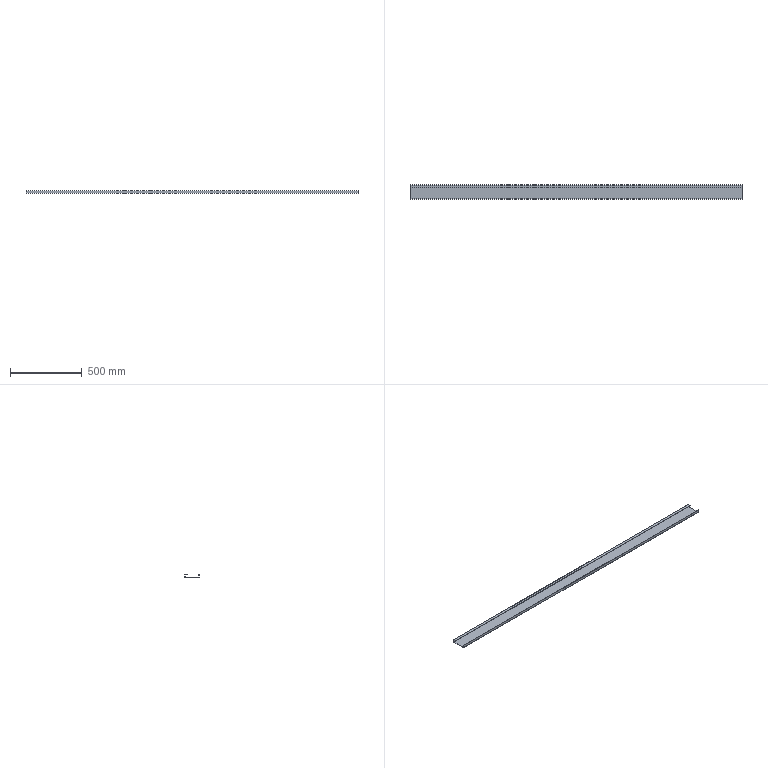Part | STEP file | 电柜通道护栏1踢脚Plate | 1 solid | 18 faces | box 2320 x 100 x 20 mm | volume 533298 mm3 | plane 12 | cylinder 6 | commonest cylinder face diameters 2 x3 5 x3
STEP:
#1=CARTESIAN_POINT('',(0.,0.,0.));
#2=DIRECTION('',(0.,0.,1.));
#3=DIRECTION('',(1.,0.,0.));
#4=AXIS2_PLACEMENT_3D('',#1,#2,#3);
#5=CARTESIAN_POINT('',(-1160.,1.5,2.5));
#6=VERTEX_POINT('',#5);
#7=CARTESIAN_POINT('',(-1160.,1.5,20.));
#8=VERTEX_POINT('',#7);
#9=CARTESIAN_POINT('',(-1160.,1.5,2.5));
#10=DIRECTION('',(0.,0.,1.));
#11=VECTOR('',#10,1.);
#12=LINE('',#9,#11);
#13=CARTESIAN_POINT('',(1160.,1.5,2.5));
#14=DIRECTION('',(0.,-1.,0.));
#15=DIRECTION('',(0.,0.,-1.));
#16=AXIS2_PLACEMENT_3D('',#13,#14,#15);
#17=PLANE('',#16);
#18=CARTESIAN_POINT('',(0.,-2320.));
#19=DIRECTION('',(-1.,0.));
#20=VECTOR('',#19,1.);
#21=LINE('',#18,#20);
#22=(GEOMETRIC_REPRESENTATION_CONTEXT(2)PARAMETRIC_REPRESENTATION_CONTEXT()REPRESENTATION_CONTEXT('',''));
#23=DEFINITIONAL_REPRESENTATION('',(#21),#22);
#24=PCURVE('',#17,#23);
#25=CARTESIAN_POINT('',(-1160.,2.5,2.5));
#26=DIRECTION('',(-1.,0.,0.));
#27=DIRECTION('',(0.,0.,1.));
#28=AXIS2_PLACEMENT_3D('',#25,#26,#27);
#29=PLANE('',#28);
#30=CARTESIAN_POINT('',(0.,-1.));
#31=DIRECTION('',(1.,0.));
#32=VECTOR('',#31,1.);
#33=LINE('',#30,#32);
#34=(GEOMETRIC_REPRESENTATION_CONTEXT(2)PARAMETRIC_REPRESENTATION_CONTEXT()REPRESENTATION_CONTEXT('',''));
#35=DEFINITIONAL_REPRESENTATION('',(#33),#34);
#36=PCURVE('',#29,#35);
#37=SURFACE_CURVE('',#12,(#24,#36),.PCURVE_S1.);
#38=EDGE_CURVE('',#6,#8,#37,.T.);
#39=ORIENTED_EDGE('',*,*,#38,.T.);
#40=CARTESIAN_POINT('',(1160.,1.5,20.));
#41=VERTEX_POINT('',#40);
#42=CARTESIAN_POINT('',(1160.,1.5,20.));
#43=DIRECTION('',(-1.,0.,0.));
#44=VECTOR('',#43,1.);
#45=LINE('',#42,#44);
#46=CARTESIAN_POINT('',(-17.5,0.));
#47=DIRECTION('',(0.,-1.));
#48=VECTOR('',#47,1.);
#49=LINE('',#46,#48);
#50=(GEOMETRIC_REPRESENTATION_CONTEXT(2)PARAMETRIC_REPRESENTATION_CONTEXT()REPRESENTATION_CONTEXT('',''));
#51=DEFINITIONAL_REPRESENTATION('',(#49),#50);
#52=PCURVE('',#17,#51);
#53=CARTESIAN_POINT('',(1160.,0.,20.));
#54=DIRECTION('',(0.,0.,1.));
#55=DIRECTION('',(1.,0.,0.));
#56=AXIS2_PLACEMENT_3D('',#53,#54,#55);
#57=PLANE('',#56);
#58=CARTESIAN_POINT('',(0.,1.5));
#59=DIRECTION('',(-1.,0.));
#60=VECTOR('',#59,1.);
#61=LINE('',#58,#60);
#62=(GEOMETRIC_REPRESENTATION_CONTEXT(2)PARAMETRIC_REPRESENTATION_CONTEXT()REPRESENTATION_CONTEXT('',''));
#63=DEFINITIONAL_REPRESENTATION('',(#61),#62);
#64=PCURVE('',#57,#63);
#65=SURFACE_CURVE('',#45,(#52,#64),.PCURVE_S1.);
#66=EDGE_CURVE('',#41,#8,#65,.T.);
#67=ORIENTED_EDGE('',*,*,#66,.F.);
#68=CARTESIAN_POINT('',(1160.,1.5,2.5));
#69=VERTEX_POINT('',#68);
#70=CARTESIAN_POINT('',(1160.,1.5,2.5));
#71=DIRECTION('',(0.,0.,1.));
#72=VECTOR('',#71,1.);
#73=LINE('',#70,#72);
#74=CARTESIAN_POINT('',(0.,0.));
#75=DIRECTION('',(-1.,0.));
#76=VECTOR('',#75,1.);
#77=LINE('',#74,#76);
#78=(GEOMETRIC_REPRESENTATION_CONTEXT(2)PARAMETRIC_REPRESENTATION_CONTEXT()REPRESENTATION_CONTEXT('',''));
#79=DEFINITIONAL_REPRESENTATION('',(#77),#78);
#80=PCURVE('',#17,#79);
#81=CARTESIAN_POINT('',(1160.,2.5,2.5));
#82=DIRECTION('',(-1.,0.,0.));
#83=DIRECTION('',(0.,0.,1.));
#84=AXIS2_PLACEMENT_3D('',#81,#82,#83);
#85=PLANE('',#84);
#86=CARTESIAN_POINT('',(0.,-1.));
#87=DIRECTION('',(1.,0.));
#88=VECTOR('',#87,1.);
#89=LINE('',#86,#88);
#90=(GEOMETRIC_REPRESENTATION_CONTEXT(2)PARAMETRIC_REPRESENTATION_CONTEXT()REPRESENTATION_CONTEXT('',''));
#91=DEFINITIONAL_REPRESENTATION('',(#89),#90);
#92=PCURVE('',#85,#91);
#93=SURFACE_CURVE('',#73,(#80,#92),.PCURVE_S1.);
#94=EDGE_CURVE('',#69,#41,#93,.T.);
#95=ORIENTED_EDGE('',*,*,#94,.F.);
#96=CARTESIAN_POINT('',(1160.,1.5,2.5));
#97=DIRECTION('',(-1.,0.,0.));
#98=VECTOR('',#97,1.);
#99=LINE('',#96,#98);
#100=CARTESIAN_POINT('',(0.,0.));
#101=DIRECTION('',(0.,-1.));
#102=VECTOR('',#101,1.);
#103=LINE('',#100,#102);
#104=(GEOMETRIC_REPRESENTATION_CONTEXT(2)PARAMETRIC_REPRESENTATION_CONTEXT()REPRESENTATION_CONTEXT('',''));
#105=DEFINITIONAL_REPRESENTATION('',(#103),#104);
#106=PCURVE('',#17,#105);
#107=CARTESIAN_POINT('',(1160.,2.5,2.5));
#108=DIRECTION('',(-1.,0.,0.));
#109=DIRECTION('',(0.,0.,1.));
#110=AXIS2_PLACEMENT_3D('',#107,#108,#109);
#111=CYLINDRICAL_SURFACE('',#110,1.);
#112=CARTESIAN_POINT('',(4.712,0.));
#113=DIRECTION('',(0.,1.));
#114=VECTOR('',#113,1.);
#115=LINE('',#112,#114);
#116=(GEOMETRIC_REPRESENTATION_CONTEXT(2)PARAMETRIC_REPRESENTATION_CONTEXT()REPRESENTATION_CONTEXT('',''));
#117=DEFINITIONAL_REPRESENTATION('',(#115),#116);
#118=PCURVE('',#111,#117);
#119=SURFACE_CURVE('',#99,(#106,#118),.PCURVE_S1.);
#120=EDGE_CURVE('',#69,#6,#119,.T.);
#121=ORIENTED_EDGE('',*,*,#120,.T.);
#122=EDGE_LOOP('',(#39,#67,#95,#121));
#123=FACE_BOUND('',#122,.T.);
#124=ADVANCED_FACE('',(#123),#17,.F.);
#125=CARTESIAN_POINT('',(-1160.,0.,20.));
#126=VERTEX_POINT('',#125);
#127=CARTESIAN_POINT('',(-1160.,0.,20.));
#128=DIRECTION('',(0.,1.,0.));
#129=VECTOR('',#128,1.);
#130=LINE('',#127,#129);
#131=CARTESIAN_POINT('',(-2320.,0.));
#132=DIRECTION('',(0.,1.));
#133=VECTOR('',#132,1.);
#134=LINE('',#131,#133);
#135=(GEOMETRIC_REPRESENTATION_CONTEXT(2)PARAMETRIC_REPRESENTATION_CONTEXT()REPRESENTATION_CONTEXT('',''));
#136=DEFINITIONAL_REPRESENTATION('',(#134),#135);
#137=PCURVE('',#57,#136);
#138=CARTESIAN_POINT('',(17.5,-2.5));
#139=DIRECTION('',(0.,1.));
#140=VECTOR('',#139,1.);
#141=LINE('',#138,#140);
#142=(GEOMETRIC_REPRESENTATION_CONTEXT(2)PARAMETRIC_REPRESENTATION_CONTEXT()REPRESENTATION_CONTEXT('',''));
#143=DEFINITIONAL_REPRESENTATION('',(#141),#142);
#144=PCURVE('',#29,#143);
#145=SURFACE_CURVE('',#130,(#137,#144),.PCURVE_S1.);
#146=EDGE_CURVE('',#126,#8,#145,.T.);
#147=ORIENTED_EDGE('',*,*,#146,.F.);
#148=CARTESIAN_POINT('',(1160.,0.,20.));
#149=VERTEX_POINT('',#148);
#150=CARTESIAN_POINT('',(1160.,0.,20.));
#151=DIRECTION('',(-1.,0.,0.));
#152=VECTOR('',#151,1.);
#153=LINE('',#150,#152);
#154=CARTESIAN_POINT('',(0.,0.));
#155=DIRECTION('',(-1.,0.));
#156=VECTOR('',#155,1.);
#157=LINE('',#154,#156);
#158=(GEOMETRIC_REPRESENTATION_CONTEXT(2)PARAMETRIC_REPRESENTATION_CONTEXT()REPRESENTATION_CONTEXT('',''));
#159=DEFINITIONAL_REPRESENTATION('',(#157),#158);
#160=PCURVE('',#57,#159);
#161=CARTESIAN_POINT('',(1160.,0.,2.5));
#162=DIRECTION('',(0.,-1.,0.));
#163=DIRECTION('',(0.,0.,-1.));
#164=AXIS2_PLACEMENT_3D('',#161,#162,#163);
#165=PLANE('',#164);
#166=CARTESIAN_POINT('',(-17.5,0.));
#167=DIRECTION('',(0.,-1.));
#168=VECTOR('',#167,1.);
#169=LINE('',#166,#168);
#170=(GEOMETRIC_REPRESENTATION_CONTEXT(2)PARAMETRIC_REPRESENTATION_CONTEXT()REPRESENTATION_CONTEXT('',''));
#171=DEFINITIONAL_REPRESENTATION('',(#169),#170);
#172=PCURVE('',#165,#171);
#173=SURFACE_CURVE('',#153,(#160,#172),.PCURVE_S1.);
#174=EDGE_CURVE('',#149,#126,#173,.T.);
#175=ORIENTED_EDGE('',*,*,#174,.F.);
#176=CARTESIAN_POINT('',(1160.,0.,20.));
#177=DIRECTION('',(0.,1.,0.));
#178=VECTOR('',#177,1.);
#179=LINE('',#176,#178);
#180=CARTESIAN_POINT('',(0.,0.));
#181=DIRECTION('',(0.,1.));
#182=VECTOR('',#181,1.);
#183=LINE('',#180,#182);
#184=(GEOMETRIC_REPRESENTATION_CONTEXT(2)PARAMETRIC_REPRESENTATION_CONTEXT()REPRESENTATION_CONTEXT('',''));
#185=DEFINITIONAL_REPRESENTATION('',(#183),#184);
#186=PCURVE('',#57,#185);
#187=CARTESIAN_POINT('',(17.5,-2.5));
#188=DIRECTION('',(0.,1.));
#189=VECTOR('',#188,1.);
#190=LINE('',#187,#189);
#191=(GEOMETRIC_REPRESENTATION_CONTEXT(2)PARAMETRIC_REPRESENTATION_CONTEXT()REPRESENTATION_CONTEXT('',''));
#192=DEFINITIONAL_REPRESENTATION('',(#190),#191);
#193=PCURVE('',#85,#192);
#194=SURFACE_CURVE('',#179,(#186,#193),.PCURVE_S1.);
#195=EDGE_CURVE('',#149,#41,#194,.T.);
#196=ORIENTED_EDGE('',*,*,#195,.T.);
#197=ORIENTED_EDGE('',*,*,#66,.T.);
#198=EDGE_LOOP('',(#147,#175,#196,#197));
#199=FACE_BOUND('',#198,.T.);
#200=ADVANCED_FACE('',(#199),#57,.T.);
#201=CARTESIAN_POINT('',(-1160.,0.,2.5));
#202=VERTEX_POINT('',#201);
#203=CARTESIAN_POINT('',(-1160.,0.,2.5));
#204=DIRECTION('',(0.,0.,1.));
#205=VECTOR('',#204,1.);
#206=LINE('',#203,#205);
#207=CARTESIAN_POINT('',(0.,-2320.));
#208=DIRECTION('',(-1.,0.));
#209=VECTOR('',#208,1.);
#210=LINE('',#207,#209);
#211=(GEOMETRIC_REPRESENTATION_CONTEXT(2)PARAMETRIC_REPRESENTATION_CONTEXT()REPRESENTATION_CONTEXT('',''));
#212=DEFINITIONAL_REPRESENTATION('',(#210),#211);
#213=PCURVE('',#165,#212);
#214=CARTESIAN_POINT('',(0.,-2.5));
#215=DIRECTION('',(1.,0.));
#216=VECTOR('',#215,1.);
#217=LINE('',#214,#216);
#218=(GEOMETRIC_REPRESENTATION_CONTEXT(2)PARAMETRIC_REPRESENTATION_CONTEXT()REPRESENTATION_CONTEXT('',''));
#219=DEFINITIONAL_REPRESENTATION('',(#217),#218);
#220=PCURVE('',#29,#219);
#221=SURFACE_CURVE('',#206,(#213,#220),.PCURVE_S1.);
#222=EDGE_CURVE('',#202,#126,#221,.T.);
#223=ORIENTED_EDGE('',*,*,#222,.F.);
#224=CARTESIAN_POINT('',(1160.,0.,2.5));
#225=VERTEX_POINT('',#224);
#226=CARTESIAN_POINT('',(1160.,0.,2.5));
#227=DIRECTION('',(-1.,0.,0.));
#228=VECTOR('',#227,1.);
#229=LINE('',#226,#228);
#230=CARTESIAN_POINT('',(0.,0.));
#231=DIRECTION('',(0.,-1.));
#232=VECTOR('',#231,1.);
#233=LINE('',#230,#232);
#234=(GEOMETRIC_REPRESENTATION_CONTEXT(2)PARAMETRIC_REPRESENTATION_CONTEXT()REPRESENTATION_CONTEXT('',''));
#235=DEFINITIONAL_REPRESENTATION('',(#233),#234);
#236=PCURVE('',#165,#235);
#237=CARTESIAN_POINT('',(1160.,2.5,2.5));
#238=DIRECTION('',(-1.,0.,0.));
#239=DIRECTION('',(0.,0.,1.));
#240=AXIS2_PLACEMENT_3D('',#237,#238,#239);
#241=CYLINDRICAL_SURFACE('',#240,2.5);
#242=CARTESIAN_POINT('',(4.712,0.));
#243=DIRECTION('',(0.,1.));
#244=VECTOR('',#243,1.);
#245=LINE('',#242,#244);
#246=(GEOMETRIC_REPRESENTATION_CONTEXT(2)PARAMETRIC_REPRESENTATION_CONTEXT()REPRESENTATION_CONTEXT('',''));
#247=DEFINITIONAL_REPRESENTATION('',(#245),#246);
#248=PCURVE('',#241,#247);
#249=SURFACE_CURVE('',#229,(#236,#248),.PCURVE_S1.);
#250=EDGE_CURVE('',#225,#202,#249,.T.);
#251=ORIENTED_EDGE('',*,*,#250,.F.);
#252=CARTESIAN_POINT('',(1160.,0.,2.5));
#253=DIRECTION('',(0.,0.,1.));
#254=VECTOR('',#253,1.);
#255=LINE('',#252,#254);
#256=CARTESIAN_POINT('',(0.,0.));
#257=DIRECTION('',(-1.,0.));
#258=VECTOR('',#257,1.);
#259=LINE('',#256,#258);
#260=(GEOMETRIC_REPRESENTATION_CONTEXT(2)PARAMETRIC_REPRESENTATION_CONTEXT()REPRESENTATION_CONTEXT('',''));
#261=DEFINITIONAL_REPRESENTATION('',(#259),#260);
#262=PCURVE('',#165,#261);
#263=CARTESIAN_POINT('',(0.,-2.5));
#264=DIRECTION('',(1.,0.));
#265=VECTOR('',#264,1.);
#266=LINE('',#263,#265);
#267=(GEOMETRIC_REPRESENTATION_CONTEXT(2)PARAMETRIC_REPRESENTATION_CONTEXT()REPRESENTATION_CONTEXT('',''));
#268=DEFINITIONAL_REPRESENTATION('',(#266),#267);
#269=PCURVE('',#85,#268);
#270=SURFACE_CURVE('',#255,(#262,#269),.PCURVE_S1.);
#271=EDGE_CURVE('',#225,#149,#270,.T.);
#272=ORIENTED_EDGE('',*,*,#271,.T.);
#273=ORIENTED_EDGE('',*,*,#174,.T.);
#274=EDGE_LOOP('',(#223,#251,#272,#273));
#275=FACE_BOUND('',#274,.T.);
#276=ADVANCED_FACE('',(#275),#165,.T.);
#277=CARTESIAN_POINT('',(-1160.,2.5,0.));
#278=VERTEX_POINT('',#277);
#279=CARTESIAN_POINT('',(-1160.,2.5,2.5));
#280=DIRECTION('',(-1.,0.,0.));
#281=DIRECTION('',(0.,0.,1.));
#282=AXIS2_PLACEMENT_3D('',#279,#280,#281);
#283=CIRCLE('',#282,2.5);
#284=CARTESIAN_POINT('',(0.,2320.));
#285=DIRECTION('',(1.,0.));
#286=VECTOR('',#285,1.);
#287=LINE('',#284,#286);
#288=(GEOMETRIC_REPRESENTATION_CONTEXT(2)PARAMETRIC_REPRESENTATION_CONTEXT()REPRESENTATION_CONTEXT('',''));
#289=DEFINITIONAL_REPRESENTATION('',(#287),#288);
#290=PCURVE('',#241,#289);
#291=CARTESIAN_POINT('',(0.,0.));
#292=DIRECTION('',(1.,0.));
#293=AXIS2_PLACEMENT_2D('',#291,#292);
#294=CIRCLE('',#293,2.5);
#295=(GEOMETRIC_REPRESENTATION_CONTEXT(2)PARAMETRIC_REPRESENTATION_CONTEXT()REPRESENTATION_CONTEXT('',''));
#296=DEFINITIONAL_REPRESENTATION('',(#294),#295);
#297=PCURVE('',#29,#296);
#298=SURFACE_CURVE('',#283,(#290,#297),.PCURVE_S1.);
#299=EDGE_CURVE('',#278,#202,#298,.T.);
#300=ORIENTED_EDGE('',*,*,#299,.F.);
#301=CARTESIAN_POINT('',(1160.,2.5,0.));
#302=VERTEX_POINT('',#301);
#303=CARTESIAN_POINT('',(1160.,2.5,0.));
#304=DIRECTION('',(-1.,0.,0.));
#305=VECTOR('',#304,1.);
#306=LINE('',#303,#305);
#307=CARTESIAN_POINT('',(3.142,0.));
#308=DIRECTION('',(0.,1.));
#309=VECTOR('',#308,1.);
#310=LINE('',#307,#309);
#311=(GEOMETRIC_REPRESENTATION_CONTEXT(2)PARAMETRIC_REPRESENTATION_CONTEXT()REPRESENTATION_CONTEXT('',''));
#312=DEFINITIONAL_REPRESENTATION('',(#310),#311);
#313=PCURVE('',#241,#312);
#314=CARTESIAN_POINT('',(1160.,2.5,0.));
#315=DIRECTION('',(0.,0.,-1.));
#316=DIRECTION('',(-1.,0.,0.));
#317=AXIS2_PLACEMENT_3D('',#314,#315,#316);
#318=PLANE('',#317);
#319=CARTESIAN_POINT('',(0.,0.));
#320=DIRECTION('',(1.,0.));
#321=VECTOR('',#320,1.);
#322=LINE('',#319,#321);
#323=(GEOMETRIC_REPRESENTATION_CONTEXT(2)PARAMETRIC_REPRESENTATION_CONTEXT()REPRESENTATION_CONTEXT('',''));
#324=DEFINITIONAL_REPRESENTATION('',(#322),#323);
#325=PCURVE('',#318,#324);
#326=SURFACE_CURVE('',#306,(#313,#325),.PCURVE_S1.);
#327=EDGE_CURVE('',#302,#278,#326,.T.);
#328=ORIENTED_EDGE('',*,*,#327,.F.);
#329=CARTESIAN_POINT('',(1160.,2.5,2.5));
#330=DIRECTION('',(-1.,0.,0.));
#331=DIRECTION('',(0.,0.,1.));
#332=AXIS2_PLACEMENT_3D('',#329,#330,#331);
#333=CIRCLE('',#332,2.5);
#334=CARTESIAN_POINT('',(0.,0.));
#335=DIRECTION('',(1.,0.));
#336=VECTOR('',#335,1.);
#337=LINE('',#334,#336);
#338=(GEOMETRIC_REPRESENTATION_CONTEXT(2)PARAMETRIC_REPRESENTATION_CONTEXT()REPRESENTATION_CONTEXT('',''));
#339=DEFINITIONAL_REPRESENTATION('',(#337),#338);
#340=PCURVE('',#241,#339);
#341=CARTESIAN_POINT('',(0.,0.));
#342=DIRECTION('',(1.,0.));
#343=AXIS2_PLACEMENT_2D('',#341,#342);
#344=CIRCLE('',#343,2.5);
#345=(GEOMETRIC_REPRESENTATION_CONTEXT(2)PARAMETRIC_REPRESENTATION_CONTEXT()REPRESENTATION_CONTEXT('',''));
#346=DEFINITIONAL_REPRESENTATION('',(#344),#345);
#347=PCURVE('',#85,#346);
#348=SURFACE_CURVE('',#333,(#340,#347),.PCURVE_S1.);
#349=EDGE_CURVE('',#302,#225,#348,.T.);
#350=ORIENTED_EDGE('',*,*,#349,.T.);
#351=ORIENTED_EDGE('',*,*,#250,.T.);
#352=EDGE_LOOP('',(#300,#328,#350,#351));
#353=FACE_BOUND('',#352,.T.);
#354=ADVANCED_FACE('',(#353),#241,.T.);
#355=CARTESIAN_POINT('',(-1160.,97.5,0.));
#356=VERTEX_POINT('',#355);
#357=CARTESIAN_POINT('',(-1160.,2.5,0.));
#358=DIRECTION('',(0.,-1.,0.));
#359=VECTOR('',#358,1.);
#360=LINE('',#357,#359);
#361=CARTESIAN_POINT('',(2320.,0.));
#362=DIRECTION('',(0.,-1.));
#363=VECTOR('',#362,1.);
#364=LINE('',#361,#363);
#365=(GEOMETRIC_REPRESENTATION_CONTEXT(2)PARAMETRIC_REPRESENTATION_CONTEXT()REPRESENTATION_CONTEXT('',''));
#366=DEFINITIONAL_REPRESENTATION('',(#364),#365);
#367=PCURVE('',#318,#366);
#368=CARTESIAN_POINT('',(-2.5,0.));
#369=DIRECTION('',(0.,-1.));
#370=VECTOR('',#369,1.);
#371=LINE('',#368,#370);
#372=(GEOMETRIC_REPRESENTATION_CONTEXT(2)PARAMETRIC_REPRESENTATION_CONTEXT()REPRESENTATION_CONTEXT('',''));
#373=DEFINITIONAL_REPRESENTATION('',(#371),#372);
#374=PCURVE('',#29,#373);
#375=SURFACE_CURVE('',#360,(#367,#374),.PCURVE_S1.);
#376=EDGE_CURVE('',#356,#278,#375,.T.);
#377=ORIENTED_EDGE('',*,*,#376,.F.);
#378=CARTESIAN_POINT('',(1160.,97.5,0.));
#379=VERTEX_POINT('',#378);
#380=CARTESIAN_POINT('',(1160.,97.5,0.));
#381=DIRECTION('',(-1.,0.,0.));
#382=VECTOR('',#381,1.);
#383=LINE('',#380,#382);
#384=CARTESIAN_POINT('',(0.,95.));
#385=DIRECTION('',(1.,0.));
#386=VECTOR('',#385,1.);
#387=LINE('',#384,#386);
#388=(GEOMETRIC_REPRESENTATION_CONTEXT(2)PARAMETRIC_REPRESENTATION_CONTEXT()REPRESENTATION_CONTEXT('',''));
#389=DEFINITIONAL_REPRESENTATION('',(#387),#388);
#390=PCURVE('',#318,#389);
#391=CARTESIAN_POINT('',(1160.,97.5,2.5));
#392=DIRECTION('',(-1.,0.,0.));
#393=DIRECTION('',(0.,0.,1.));
#394=AXIS2_PLACEMENT_3D('',#391,#392,#393);
#395=CYLINDRICAL_SURFACE('',#394,2.5);
#396=CARTESIAN_POINT('',(3.142,0.));
#397=DIRECTION('',(0.,1.));
#398=VECTOR('',#397,1.);
#399=LINE('',#396,#398);
#400=(GEOMETRIC_REPRESENTATION_CONTEXT(2)PARAMETRIC_REPRESENTATION_CONTEXT()REPRESENTATION_CONTEXT('',''));
#401=DEFINITIONAL_REPRESENTATION('',(#399),#400);
#402=PCURVE('',#395,#401);
#403=SURFACE_CURVE('',#383,(#390,#402),.PCURVE_S1.);
#404=EDGE_CURVE('',#379,#356,#403,.T.);
#405=ORIENTED_EDGE('',*,*,#404,.F.);
#406=CARTESIAN_POINT('',(1160.,2.5,0.));
#407=DIRECTION('',(0.,-1.,0.));
#408=VECTOR('',#407,1.);
#409=LINE('',#406,#408);
#410=CARTESIAN_POINT('',(0.,0.));
#411=DIRECTION('',(0.,-1.));
#412=VECTOR('',#411,1.);
#413=LINE('',#410,#412);
#414=(GEOMETRIC_REPRESENTATION_CONTEXT(2)PARAMETRIC_REPRESENTATION_CONTEXT()REPRESENTATION_CONTEXT('',''));
#415=DEFINITIONAL_REPRESENTATION('',(#413),#414);
#416=PCURVE('',#318,#415);
#417=CARTESIAN_POINT('',(-2.5,0.));
#418=DIRECTION('',(0.,-1.));
#419=VECTOR('',#418,1.);
#420=LINE('',#417,#419);
#421=(GEOMETRIC_REPRESENTATION_CONTEXT(2)PARAMETRIC_REPRESENTATION_CONTEXT()REPRESENTATION_CONTEXT('',''));
#422=DEFINITIONAL_REPRESENTATION('',(#420),#421);
#423=PCURVE('',#85,#422);
#424=SURFACE_CURVE('',#409,(#416,#423),.PCURVE_S1.);
#425=EDGE_CURVE('',#379,#302,#424,.T.);
#426=ORIENTED_EDGE('',*,*,#425,.T.);
#427=ORIENTED_EDGE('',*,*,#327,.T.);
#428=EDGE_LOOP('',(#377,#405,#426,#427));
#429=FACE_BOUND('',#428,.T.);
#430=ADVANCED_FACE('',(#429),#318,.T.);
#431=CARTESIAN_POINT('',(-1160.,100.,2.5));
#432=VERTEX_POINT('',#431);
#433=CARTESIAN_POINT('',(-1160.,97.5,2.5));
#434=DIRECTION('',(-1.,0.,0.));
#435=DIRECTION('',(0.,0.,-1.));
#436=AXIS2_PLACEMENT_3D('',#433,#434,#435);
#437=CIRCLE('',#436,2.5);
#438=CARTESIAN_POINT('',(-3.142,2320.));
#439=DIRECTION('',(1.,0.));
#440=VECTOR('',#439,1.);
#441=LINE('',#438,#440);
#442=(GEOMETRIC_REPRESENTATION_CONTEXT(2)PARAMETRIC_REPRESENTATION_CONTEXT()REPRESENTATION_CONTEXT('',''));
#443=DEFINITIONAL_REPRESENTATION('',(#441),#442);
#444=PCURVE('',#395,#443);
#445=CARTESIAN_POINT('',(0.,95.));
#446=DIRECTION('',(-1.,0.));
#447=AXIS2_PLACEMENT_2D('',#445,#446);
#448=CIRCLE('',#447,2.5);
#449=(GEOMETRIC_REPRESENTATION_CONTEXT(2)PARAMETRIC_REPRESENTATION_CONTEXT()REPRESENTATION_CONTEXT('',''));
#450=DEFINITIONAL_REPRESENTATION('',(#448),#449);
#451=PCURVE('',#29,#450);
#452=SURFACE_CURVE('',#437,(#444,#451),.PCURVE_S1.);
#453=EDGE_CURVE('',#432,#356,#452,.T.);
#454=ORIENTED_EDGE('',*,*,#453,.F.);
#455=CARTESIAN_POINT('',(1160.,100.,2.5));
#456=VERTEX_POINT('',#455);
#457=CARTESIAN_POINT('',(1160.,100.,2.5));
#458=DIRECTION('',(-1.,0.,0.));
#459=VECTOR('',#458,1.);
#460=LINE('',#457,#459);
#461=CARTESIAN_POINT('',(1.571,0.));
#462=DIRECTION('',(0.,1.));
#463=VECTOR('',#462,1.);
#464=LINE('',#461,#463);
#465=(GEOMETRIC_REPRESENTATION_CONTEXT(2)PARAMETRIC_REPRESENTATION_CONTEXT()REPRESENTATION_CONTEXT('',''));
#466=DEFINITIONAL_REPRESENTATION('',(#464),#465);
#467=PCURVE('',#395,#466);
#468=CARTESIAN_POINT('',(1160.,100.,2.5));
#469=DIRECTION('',(0.,1.,0.));
#470=DIRECTION('',(0.,0.,1.));
#471=AXIS2_PLACEMENT_3D('',#468,#469,#470);
#472=PLANE('',#471);
#473=CARTESIAN_POINT('',(0.,0.));
#474=DIRECTION('',(0.,-1.));
#475=VECTOR('',#474,1.);
#476=LINE('',#473,#475);
#477=(GEOMETRIC_REPRESENTATION_CONTEXT(2)PARAMETRIC_REPRESENTATION_CONTEXT()REPRESENTATION_CONTEXT('',''));
#478=DEFINITIONAL_REPRESENTATION('',(#476),#477);
#479=PCURVE('',#472,#478);
#480=SURFACE_CURVE('',#460,(#467,#479),.PCURVE_S1.);
#481=EDGE_CURVE('',#456,#432,#480,.T.);
#482=ORIENTED_EDGE('',*,*,#481,.F.);
#483=CARTESIAN_POINT('',(1160.,97.5,2.5));
#484=DIRECTION('',(-1.,0.,0.));
#485=DIRECTION('',(0.,0.,-1.));
#486=AXIS2_PLACEMENT_3D('',#483,#484,#485);
#487=CIRCLE('',#486,2.5);
#488=CARTESIAN_POINT('',(-3.142,0.));
#489=DIRECTION('',(1.,0.));
#490=VECTOR('',#489,1.);
#491=LINE('',#488,#490);
#492=(GEOMETRIC_REPRESENTATION_CONTEXT(2)PARAMETRIC_REPRESENTATION_CONTEXT()REPRESENTATION_CONTEXT('',''));
#493=DEFINITIONAL_REPRESENTATION('',(#491),#492);
#494=PCURVE('',#395,#493);
#495=CARTESIAN_POINT('',(0.,95.));
#496=DIRECTION('',(-1.,0.));
#497=AXIS2_PLACEMENT_2D('',#495,#496);
#498=CIRCLE('',#497,2.5);
#499=(GEOMETRIC_REPRESENTATION_CONTEXT(2)PARAMETRIC_REPRESENTATION_CONTEXT()REPRESENTATION_CONTEXT('',''));
#500=DEFINITIONAL_REPRESENTATION('',(#498),#499);
#501=PCURVE('',#85,#500);
#502=SURFACE_CURVE('',#487,(#494,#501),.PCURVE_S1.);
#503=EDGE_CURVE('',#456,#379,#502,.T.);
#504=ORIENTED_EDGE('',*,*,#503,.T.);
#505=ORIENTED_EDGE('',*,*,#404,.T.);
#506=EDGE_LOOP('',(#454,#482,#504,#505));
#507=FACE_BOUND('',#506,.T.);
#508=ADVANCED_FACE('',(#507),#395,.T.);
#509=CARTESIAN_POINT('',(-1160.,100.,17.5));
#510=VERTEX_POINT('',#509);
#511=CARTESIAN_POINT('',(-1160.,100.,2.5));
#512=DIRECTION('',(0.,0.,-1.));
#513=VECTOR('',#512,1.);
#514=LINE('',#511,#513);
#515=CARTESIAN_POINT('',(0.,-2320.));
#516=DIRECTION('',(-1.,0.));
#517=VECTOR('',#516,1.);
#518=LINE('',#515,#517);
#519=(GEOMETRIC_REPRESENTATION_CONTEXT(2)PARAMETRIC_REPRESENTATION_CONTEXT()REPRESENTATION_CONTEXT('',''));
#520=DEFINITIONAL_REPRESENTATION('',(#518),#519);
#521=PCURVE('',#472,#520);
#522=CARTESIAN_POINT('',(0.,97.5));
#523=DIRECTION('',(-1.,0.));
#524=VECTOR('',#523,1.);
#525=LINE('',#522,#524);
#526=(GEOMETRIC_REPRESENTATION_CONTEXT(2)PARAMETRIC_REPRESENTATION_CONTEXT()REPRESENTATION_CONTEXT('',''));
#527=DEFINITIONAL_REPRESENTATION('',(#525),#526);
#528=PCURVE('',#29,#527);
#529=SURFACE_CURVE('',#514,(#521,#528),.PCURVE_S1.);
#530=EDGE_CURVE('',#510,#432,#529,.T.);
#531=ORIENTED_EDGE('',*,*,#530,.F.);
#532=CARTESIAN_POINT('',(1160.,100.,17.5));
#533=VERTEX_POINT('',#532);
#534=CARTESIAN_POINT('',(1160.,100.,17.5));
#535=DIRECTION('',(-1.,0.,0.));
#536=VECTOR('',#535,1.);
#537=LINE('',#534,#536);
#538=CARTESIAN_POINT('',(15.,0.));
#539=DIRECTION('',(0.,-1.));
#540=VECTOR('',#539,1.);
#541=LINE('',#538,#540);
#542=(GEOMETRIC_REPRESENTATION_CONTEXT(2)PARAMETRIC_REPRESENTATION_CONTEXT()REPRESENTATION_CONTEXT('',''));
#543=DEFINITIONAL_REPRESENTATION('',(#541),#542);
#544=PCURVE('',#472,#543);
#545=CARTESIAN_POINT('',(1160.,97.5,17.5));
#546=DIRECTION('',(-1.,0.,0.));
#547=DIRECTION('',(0.,0.,1.));
#548=AXIS2_PLACEMENT_3D('',#545,#546,#547);
#549=CYLINDRICAL_SURFACE('',#548,2.5);
#550=CARTESIAN_POINT('',(1.571,0.));
#551=DIRECTION('',(0.,1.));
#552=VECTOR('',#551,1.);
#553=LINE('',#550,#552);
#554=(GEOMETRIC_REPRESENTATION_CONTEXT(2)PARAMETRIC_REPRESENTATION_CONTEXT()REPRESENTATION_CONTEXT('',''));
#555=DEFINITIONAL_REPRESENTATION('',(#553),#554);
#556=PCURVE('',#549,#555);
#557=SURFACE_CURVE('',#537,(#544,#556),.PCURVE_S1.);
#558=EDGE_CURVE('',#533,#510,#557,.T.);
#559=ORIENTED_EDGE('',*,*,#558,.F.);
#560=CARTESIAN_POINT('',(1160.,100.,2.5));
#561=DIRECTION('',(0.,0.,-1.));
#562=VECTOR('',#561,1.);
#563=LINE('',#560,#562);
#564=CARTESIAN_POINT('',(0.,0.));
#565=DIRECTION('',(-1.,0.));
#566=VECTOR('',#565,1.);
#567=LINE('',#564,#566);
#568=(GEOMETRIC_REPRESENTATION_CONTEXT(2)PARAMETRIC_REPRESENTATION_CONTEXT()REPRESENTATION_CONTEXT('',''));
#569=DEFINITIONAL_REPRESENTATION('',(#567),#568);
#570=PCURVE('',#472,#569);
#571=CARTESIAN_POINT('',(0.,97.5));
#572=DIRECTION('',(-1.,0.));
#573=VECTOR('',#572,1.);
#574=LINE('',#571,#573);
#575=(GEOMETRIC_REPRESENTATION_CONTEXT(2)PARAMETRIC_REPRESENTATION_CONTEXT()REPRESENTATION_CONTEXT('',''));
#576=DEFINITIONAL_REPRESENTATION('',(#574),#575);
#577=PCURVE('',#85,#576);
#578=SURFACE_CURVE('',#563,(#570,#577),.PCURVE_S1.);
#579=EDGE_CURVE('',#533,#456,#578,.T.);
#580=ORIENTED_EDGE('',*,*,#579,.T.);
#581=ORIENTED_EDGE('',*,*,#481,.T.);
#582=EDGE_LOOP('',(#531,#559,#580,#581));
#583=FACE_BOUND('',#582,.T.);
#584=ADVANCED_FACE('',(#583),#472,.T.);
#585=CARTESIAN_POINT('',(-1160.,97.5,20.));
#586=VERTEX_POINT('',#585);
#587=CARTESIAN_POINT('',(-1160.,97.5,17.5));
#588=DIRECTION('',(-1.,0.,0.));
#589=DIRECTION('',(0.,0.,-1.));
#590=AXIS2_PLACEMENT_3D('',#587,#588,#589);
#591=CIRCLE('',#590,2.5);
#592=CARTESIAN_POINT('',(-3.142,2320.));
#593=DIRECTION('',(1.,0.));
#594=VECTOR('',#593,1.);
#595=LINE('',#592,#594);
#596=(GEOMETRIC_REPRESENTATION_CONTEXT(2)PARAMETRIC_REPRESENTATION_CONTEXT()REPRESENTATION_CONTEXT('',''));
#597=DEFINITIONAL_REPRESENTATION('',(#595),#596);
#598=PCURVE('',#549,#597);
#599=CARTESIAN_POINT('',(15.,95.));
#600=DIRECTION('',(-1.,0.));
#601=AXIS2_PLACEMENT_2D('',#599,#600);
#602=CIRCLE('',#601,2.5);
#603=(GEOMETRIC_REPRESENTATION_CONTEXT(2)PARAMETRIC_REPRESENTATION_CONTEXT()REPRESENTATION_CONTEXT('',''));
#604=DEFINITIONAL_REPRESENTATION('',(#602),#603);
#605=PCURVE('',#29,#604);
#606=SURFACE_CURVE('',#591,(#598,#605),.PCURVE_S1.);
#607=EDGE_CURVE('',#586,#510,#606,.T.);
#608=ORIENTED_EDGE('',*,*,#607,.F.);
#609=CARTESIAN_POINT('',(1160.,97.5,20.));
#610=VERTEX_POINT('',#609);
#611=CARTESIAN_POINT('',(1160.,97.5,20.));
#612=DIRECTION('',(-1.,0.,0.));
#613=VECTOR('',#612,1.);
#614=LINE('',#611,#613);
#615=CARTESIAN_POINT('',(0.,0.));
#616=DIRECTION('',(0.,1.));
#617=VECTOR('',#616,1.);
#618=LINE('',#615,#617);
#619=(GEOMETRIC_REPRESENTATION_CONTEXT(2)PARAMETRIC_REPRESENTATION_CONTEXT()REPRESENTATION_CONTEXT('',''));
#620=DEFINITIONAL_REPRESENTATION('',(#618),#619);
#621=PCURVE('',#549,#620);
#622=CARTESIAN_POINT('',(1160.,97.5,20.));
#623=DIRECTION('',(0.,0.,1.));
#624=DIRECTION('',(1.,0.,0.));
#625=AXIS2_PLACEMENT_3D('',#622,#623,#624);
#626=PLANE('',#625);
#627=CARTESIAN_POINT('',(0.,0.));
#628=DIRECTION('',(-1.,0.));
#629=VECTOR('',#628,1.);
#630=LINE('',#627,#629);
#631=(GEOMETRIC_REPRESENTATION_CONTEXT(2)PARAMETRIC_REPRESENTATION_CONTEXT()REPRESENTATION_CONTEXT('',''));
#632=DEFINITIONAL_REPRESENTATION('',(#630),#631);
#633=PCURVE('',#626,#632);
#634=SURFACE_CURVE('',#614,(#621,#633),.PCURVE_S1.);
#635=EDGE_CURVE('',#610,#586,#634,.T.);
#636=ORIENTED_EDGE('',*,*,#635,.F.);
#637=CARTESIAN_POINT('',(1160.,97.5,17.5));
#638=DIRECTION('',(-1.,0.,0.));
#639=DIRECTION('',(0.,0.,-1.));
#640=AXIS2_PLACEMENT_3D('',#637,#638,#639);
#641=CIRCLE('',#640,2.5);
#642=CARTESIAN_POINT('',(-3.142,0.));
#643=DIRECTION('',(1.,0.));
#644=VECTOR('',#643,1.);
#645=LINE('',#642,#644);
#646=(GEOMETRIC_REPRESENTATION_CONTEXT(2)PARAMETRIC_REPRESENTATION_CONTEXT()REPRESENTATION_CONTEXT('',''));
#647=DEFINITIONAL_REPRESENTATION('',(#645),#646);
#648=PCURVE('',#549,#647);
#649=CARTESIAN_POINT('',(15.,95.));
#650=DIRECTION('',(-1.,0.));
#651=AXIS2_PLACEMENT_2D('',#649,#650);
#652=CIRCLE('',#651,2.5);
#653=(GEOMETRIC_REPRESENTATION_CONTEXT(2)PARAMETRIC_REPRESENTATION_CONTEXT()REPRESENTATION_CONTEXT('',''));
#654=DEFINITIONAL_REPRESENTATION('',(#652),#653);
#655=PCURVE('',#85,#654);
#656=SURFACE_CURVE('',#641,(#648,#655),.PCURVE_S1.);
#657=EDGE_CURVE('',#610,#533,#656,.T.);
#658=ORIENTED_EDGE('',*,*,#657,.T.);
#659=ORIENTED_EDGE('',*,*,#558,.T.);
#660=EDGE_LOOP('',(#608,#636,#658,#659));
#661=FACE_BOUND('',#660,.T.);
#662=ADVANCED_FACE('',(#661),#549,.T.);
#663=CARTESIAN_POINT('',(-1160.,80.,20.));
#664=VERTEX_POINT('',#663);
#665=CARTESIAN_POINT('',(-1160.,97.5,20.));
#666=DIRECTION('',(0.,1.,0.));
#667=VECTOR('',#666,1.);
#668=LINE('',#665,#667);
#669=CARTESIAN_POINT('',(-2320.,0.));
#670=DIRECTION('',(0.,1.));
#671=VECTOR('',#670,1.);
#672=LINE('',#669,#671);
#673=(GEOMETRIC_REPRESENTATION_CONTEXT(2)PARAMETRIC_REPRESENTATION_CONTEXT()REPRESENTATION_CONTEXT('',''));
#674=DEFINITIONAL_REPRESENTATION('',(#672),#673);
#675=PCURVE('',#626,#674);
#676=CARTESIAN_POINT('',(17.5,95.));
#677=DIRECTION('',(0.,1.));
#678=VECTOR('',#677,1.);
#679=LINE('',#676,#678);
#680=(GEOMETRIC_REPRESENTATION_CONTEXT(2)PARAMETRIC_REPRESENTATION_CONTEXT()REPRESENTATION_CONTEXT('',''));
#681=DEFINITIONAL_REPRESENTATION('',(#679),#680);
#682=PCURVE('',#29,#681);
#683=SURFACE_CURVE('',#668,(#675,#682),.PCURVE_S1.);
#684=EDGE_CURVE('',#664,#586,#683,.T.);
#685=ORIENTED_EDGE('',*,*,#684,.F.);
#686=CARTESIAN_POINT('',(1160.,80.,20.));
#687=VERTEX_POINT('',#686);
#688=CARTESIAN_POINT('',(1160.,80.,20.));
#689=DIRECTION('',(-1.,0.,0.));
#690=VECTOR('',#689,1.);
#691=LINE('',#688,#690);
#692=CARTESIAN_POINT('',(0.,-17.5));
#693=DIRECTION('',(-1.,0.));
#694=VECTOR('',#693,1.);
#695=LINE('',#692,#694);
#696=(GEOMETRIC_REPRESENTATION_CONTEXT(2)PARAMETRIC_REPRESENTATION_CONTEXT()REPRESENTATION_CONTEXT('',''));
#697=DEFINITIONAL_REPRESENTATION('',(#695),#696);
#698=PCURVE('',#626,#697);
#699=CARTESIAN_POINT('',(1160.,80.,18.5));
#700=DIRECTION('',(0.,-1.,0.));
#701=DIRECTION('',(0.,0.,-1.));
#702=AXIS2_PLACEMENT_3D('',#699,#700,#701);
#703=PLANE('',#702);
#704=CARTESIAN_POINT('',(-1.5,0.));
#705=DIRECTION('',(0.,-1.));
#706=VECTOR('',#705,1.);
#707=LINE('',#704,#706);
#708=(GEOMETRIC_REPRESENTATION_CONTEXT(2)PARAMETRIC_REPRESENTATION_CONTEXT()REPRESENTATION_CONTEXT('',''));
#709=DEFINITIONAL_REPRESENTATION('',(#707),#708);
#710=PCURVE('',#703,#709);
#711=SURFACE_CURVE('',#691,(#698,#710),.PCURVE_S1.);
#712=EDGE_CURVE('',#687,#664,#711,.T.);
#713=ORIENTED_EDGE('',*,*,#712,.F.);
#714=CARTESIAN_POINT('',(1160.,97.5,20.));
#715=DIRECTION('',(0.,1.,0.));
#716=VECTOR('',#715,1.);
#717=LINE('',#714,#716);
#718=CARTESIAN_POINT('',(0.,0.));
#719=DIRECTION('',(0.,1.));
#720=VECTOR('',#719,1.);
#721=LINE('',#718,#720);
#722=(GEOMETRIC_REPRESENTATION_CONTEXT(2)PARAMETRIC_REPRESENTATION_CONTEXT()REPRESENTATION_CONTEXT('',''));
#723=DEFINITIONAL_REPRESENTATION('',(#721),#722);
#724=PCURVE('',#626,#723);
#725=CARTESIAN_POINT('',(17.5,95.));
#726=DIRECTION('',(0.,1.));
#727=VECTOR('',#726,1.);
#728=LINE('',#725,#727);
#729=(GEOMETRIC_REPRESENTATION_CONTEXT(2)PARAMETRIC_REPRESENTATION_CONTEXT()REPRESENTATION_CONTEXT('',''));
#730=DEFINITIONAL_REPRESENTATION('',(#728),#729);
#731=PCURVE('',#85,#730);
#732=SURFACE_CURVE('',#717,(#724,#731),.PCURVE_S1.);
#733=EDGE_CURVE('',#687,#610,#732,.T.);
#734=ORIENTED_EDGE('',*,*,#733,.T.);
#735=ORIENTED_EDGE('',*,*,#635,.T.);
#736=EDGE_LOOP('',(#685,#713,#734,#735));
#737=FACE_BOUND('',#736,.T.);
#738=ADVANCED_FACE('',(#737),#626,.T.);
#739=CARTESIAN_POINT('',(-1160.,80.,18.5));
#740=VERTEX_POINT('',#739);
#741=CARTESIAN_POINT('',(-1160.,80.,18.5));
#742=DIRECTION('',(0.,0.,1.));
#743=VECTOR('',#742,1.);
#744=LINE('',#741,#743);
#745=CARTESIAN_POINT('',(0.,-2320.));
#746=DIRECTION('',(-1.,0.));
#747=VECTOR('',#746,1.);
#748=LINE('',#745,#747);
#749=(GEOMETRIC_REPRESENTATION_CONTEXT(2)PARAMETRIC_REPRESENTATION_CONTEXT()REPRESENTATION_CONTEXT('',''));
#750=DEFINITIONAL_REPRESENTATION('',(#748),#749);
#751=PCURVE('',#703,#750);
#752=CARTESIAN_POINT('',(16.,77.5));
#753=DIRECTION('',(1.,0.));
#754=VECTOR('',#753,1.);
#755=LINE('',#752,#754);
#756=(GEOMETRIC_REPRESENTATION_CONTEXT(2)PARAMETRIC_REPRESENTATION_CONTEXT()REPRESENTATION_CONTEXT('',''));
#757=DEFINITIONAL_REPRESENTATION('',(#755),#756);
#758=PCURVE('',#29,#757);
#759=SURFACE_CURVE('',#744,(#751,#758),.PCURVE_S1.);
#760=EDGE_CURVE('',#740,#664,#759,.T.);
#761=ORIENTED_EDGE('',*,*,#760,.F.);
#762=CARTESIAN_POINT('',(1160.,80.,18.5));
#763=VERTEX_POINT('',#762);
#764=CARTESIAN_POINT('',(1160.,80.,18.5));
#765=DIRECTION('',(-1.,0.,0.));
#766=VECTOR('',#765,1.);
#767=LINE('',#764,#766);
#768=CARTESIAN_POINT('',(0.,0.));
#769=DIRECTION('',(0.,-1.));
#770=VECTOR('',#769,1.);
#771=LINE('',#768,#770);
#772=(GEOMETRIC_REPRESENTATION_CONTEXT(2)PARAMETRIC_REPRESENTATION_CONTEXT()REPRESENTATION_CONTEXT('',''));
#773=DEFINITIONAL_REPRESENTATION('',(#771),#772);
#774=PCURVE('',#703,#773);
#775=CARTESIAN_POINT('',(1160.,97.5,18.5));
#776=DIRECTION('',(0.,0.,1.));
#777=DIRECTION('',(1.,0.,0.));
#778=AXIS2_PLACEMENT_3D('',#775,#776,#777);
#779=PLANE('',#778);
#780=CARTESIAN_POINT('',(0.,-17.5));
#781=DIRECTION('',(-1.,0.));
#782=VECTOR('',#781,1.);
#783=LINE('',#780,#782);
#784=(GEOMETRIC_REPRESENTATION_CONTEXT(2)PARAMETRIC_REPRESENTATION_CONTEXT()REPRESENTATION_CONTEXT('',''));
#785=DEFINITIONAL_REPRESENTATION('',(#783),#784);
#786=PCURVE('',#779,#785);
#787=SURFACE_CURVE('',#767,(#774,#786),.PCURVE_S1.);
#788=EDGE_CURVE('',#763,#740,#787,.T.);
#789=ORIENTED_EDGE('',*,*,#788,.F.);
#790=CARTESIAN_POINT('',(1160.,80.,18.5));
#791=DIRECTION('',(0.,0.,1.));
#792=VECTOR('',#791,1.);
#793=LINE('',#790,#792);
#794=CARTESIAN_POINT('',(0.,0.));
#795=DIRECTION('',(-1.,0.));
#796=VECTOR('',#795,1.);
#797=LINE('',#794,#796);
#798=(GEOMETRIC_REPRESENTATION_CONTEXT(2)PARAMETRIC_REPRESENTATION_CONTEXT()REPRESENTATION_CONTEXT('',''));
#799=DEFINITIONAL_REPRESENTATION('',(#797),#798);
#800=PCURVE('',#703,#799);
#801=CARTESIAN_POINT('',(16.,77.5));
#802=DIRECTION('',(1.,0.));
#803=VECTOR('',#802,1.);
#804=LINE('',#801,#803);
#805=(GEOMETRIC_REPRESENTATION_CONTEXT(2)PARAMETRIC_REPRESENTATION_CONTEXT()REPRESENTATION_CONTEXT('',''));
#806=DEFINITIONAL_REPRESENTATION('',(#804),#805);
#807=PCURVE('',#85,#806);
#808=SURFACE_CURVE('',#793,(#800,#807),.PCURVE_S1.);
#809=EDGE_CURVE('',#763,#687,#808,.T.);
#810=ORIENTED_EDGE('',*,*,#809,.T.);
#811=ORIENTED_EDGE('',*,*,#712,.T.);
#812=EDGE_LOOP('',(#761,#789,#810,#811));
#813=FACE_BOUND('',#812,.T.);
#814=ADVANCED_FACE('',(#813),#703,.T.);
#815=CARTESIAN_POINT('',(-1160.,97.5,18.5));
#816=VERTEX_POINT('',#815);
#817=CARTESIAN_POINT('',(-1160.,97.5,18.5));
#818=DIRECTION('',(0.,1.,0.));
#819=VECTOR('',#818,1.);
#820=LINE('',#817,#819);
#821=CARTESIAN_POINT('',(-2320.,0.));
#822=DIRECTION('',(0.,1.));
#823=VECTOR('',#822,1.);
#824=LINE('',#821,#823);
#825=(GEOMETRIC_REPRESENTATION_CONTEXT(2)PARAMETRIC_REPRESENTATION_CONTEXT()REPRESENTATION_CONTEXT('',''));
#826=DEFINITIONAL_REPRESENTATION('',(#824),#825);
#827=PCURVE('',#779,#826);
#828=CARTESIAN_POINT('',(16.,95.));
#829=DIRECTION('',(0.,1.));
#830=VECTOR('',#829,1.);
#831=LINE('',#828,#830);
#832=(GEOMETRIC_REPRESENTATION_CONTEXT(2)PARAMETRIC_REPRESENTATION_CONTEXT()REPRESENTATION_CONTEXT('',''));
#833=DEFINITIONAL_REPRESENTATION('',(#831),#832);
#834=PCURVE('',#29,#833);
#835=SURFACE_CURVE('',#820,(#827,#834),.PCURVE_S1.);
#836=EDGE_CURVE('',#740,#816,#835,.T.);
#837=ORIENTED_EDGE('',*,*,#836,.T.);
#838=CARTESIAN_POINT('',(1160.,97.5,18.5));
#839=VERTEX_POINT('',#838);
#840=CARTESIAN_POINT('',(1160.,97.5,18.5));
#841=DIRECTION('',(-1.,0.,0.));
#842=VECTOR('',#841,1.);
#843=LINE('',#840,#842);
#844=CARTESIAN_POINT('',(0.,0.));
#845=DIRECTION('',(-1.,0.));
#846=VECTOR('',#845,1.);
#847=LINE('',#844,#846);
#848=(GEOMETRIC_REPRESENTATION_CONTEXT(2)PARAMETRIC_REPRESENTATION_CONTEXT()REPRESENTATION_CONTEXT('',''));
#849=DEFINITIONAL_REPRESENTATION('',(#847),#848);
#850=PCURVE('',#779,#849);
#851=CARTESIAN_POINT('',(1160.,97.5,17.5));
#852=DIRECTION('',(-1.,0.,0.));
#853=DIRECTION('',(0.,0.,1.));
#854=AXIS2_PLACEMENT_3D('',#851,#852,#853);
#855=CYLINDRICAL_SURFACE('',#854,1.);
#856=CARTESIAN_POINT('',(0.,0.));
#857=DIRECTION('',(0.,1.));
#858=VECTOR('',#857,1.);
#859=LINE('',#856,#858);
#860=(GEOMETRIC_REPRESENTATION_CONTEXT(2)PARAMETRIC_REPRESENTATION_CONTEXT()REPRESENTATION_CONTEXT('',''));
#861=DEFINITIONAL_REPRESENTATION('',(#859),#860);
#862=PCURVE('',#855,#861);
#863=SURFACE_CURVE('',#843,(#850,#862),.PCURVE_S1.);
#864=EDGE_CURVE('',#839,#816,#863,.T.);
#865=ORIENTED_EDGE('',*,*,#864,.F.);
#866=CARTESIAN_POINT('',(1160.,97.5,18.5));
#867=DIRECTION('',(0.,1.,0.));
#868=VECTOR('',#867,1.);
#869=LINE('',#866,#868);
#870=CARTESIAN_POINT('',(0.,0.));
#871=DIRECTION('',(0.,1.));
#872=VECTOR('',#871,1.);
#873=LINE('',#870,#872);
#874=(GEOMETRIC_REPRESENTATION_CONTEXT(2)PARAMETRIC_REPRESENTATION_CONTEXT()REPRESENTATION_CONTEXT('',''));
#875=DEFINITIONAL_REPRESENTATION('',(#873),#874);
#876=PCURVE('',#779,#875);
#877=CARTESIAN_POINT('',(16.,95.));
#878=DIRECTION('',(0.,1.));
#879=VECTOR('',#878,1.);
#880=LINE('',#877,#879);
#881=(GEOMETRIC_REPRESENTATION_CONTEXT(2)PARAMETRIC_REPRESENTATION_CONTEXT()REPRESENTATION_CONTEXT('',''));
#882=DEFINITIONAL_REPRESENTATION('',(#880),#881);
#883=PCURVE('',#85,#882);
#884=SURFACE_CURVE('',#869,(#876,#883),.PCURVE_S1.);
#885=EDGE_CURVE('',#763,#839,#884,.T.);
#886=ORIENTED_EDGE('',*,*,#885,.F.);
#887=ORIENTED_EDGE('',*,*,#788,.T.);
#888=EDGE_LOOP('',(#837,#865,#886,#887));
#889=FACE_BOUND('',#888,.T.);
#890=ADVANCED_FACE('',(#889),#779,.F.);
#891=ORIENTED_EDGE('',*,*,#864,.F.);
#892=CARTESIAN_POINT('',(1160.,98.5,17.5));
#893=VERTEX_POINT('',#892);
#894=CARTESIAN_POINT('',(1160.,97.5,17.5));
#895=DIRECTION('',(-1.,0.,0.));
#896=DIRECTION('',(0.,0.,-1.));
#897=AXIS2_PLACEMENT_3D('',#894,#895,#896);
#898=CIRCLE('',#897,1.);
#899=CARTESIAN_POINT('',(-3.142,0.));
#900=DIRECTION('',(1.,0.));
#901=VECTOR('',#900,1.);
#902=LINE('',#899,#901);
#903=(GEOMETRIC_REPRESENTATION_CONTEXT(2)PARAMETRIC_REPRESENTATION_CONTEXT()REPRESENTATION_CONTEXT('',''));
#904=DEFINITIONAL_REPRESENTATION('',(#902),#903);
#905=PCURVE('',#855,#904);
#906=CARTESIAN_POINT('',(15.,95.));
#907=DIRECTION('',(-1.,0.));
#908=AXIS2_PLACEMENT_2D('',#906,#907);
#909=CIRCLE('',#908,1.);
#910=(GEOMETRIC_REPRESENTATION_CONTEXT(2)PARAMETRIC_REPRESENTATION_CONTEXT()REPRESENTATION_CONTEXT('',''));
#911=DEFINITIONAL_REPRESENTATION('',(#909),#910);
#912=PCURVE('',#85,#911);
#913=SURFACE_CURVE('',#898,(#905,#912),.PCURVE_S1.);
#914=EDGE_CURVE('',#839,#893,#913,.T.);
#915=ORIENTED_EDGE('',*,*,#914,.T.);
#916=CARTESIAN_POINT('',(-1160.,98.5,17.5));
#917=VERTEX_POINT('',#916);
#918=CARTESIAN_POINT('',(1160.,98.5,17.5));
#919=DIRECTION('',(-1.,0.,0.));
#920=VECTOR('',#919,1.);
#921=LINE('',#918,#920);
#922=CARTESIAN_POINT('',(1.571,0.));
#923=DIRECTION('',(0.,1.));
#924=VECTOR('',#923,1.);
#925=LINE('',#922,#924);
#926=(GEOMETRIC_REPRESENTATION_CONTEXT(2)PARAMETRIC_REPRESENTATION_CONTEXT()REPRESENTATION_CONTEXT('',''));
#927=DEFINITIONAL_REPRESENTATION('',(#925),#926);
#928=PCURVE('',#855,#927);
#929=CARTESIAN_POINT('',(1160.,98.5,2.5));
#930=DIRECTION('',(0.,1.,0.));
#931=DIRECTION('',(0.,0.,1.));
#932=AXIS2_PLACEMENT_3D('',#929,#930,#931);
#933=PLANE('',#932);
#934=CARTESIAN_POINT('',(15.,0.));
#935=DIRECTION('',(0.,-1.));
#936=VECTOR('',#935,1.);
#937=LINE('',#934,#936);
#938=(GEOMETRIC_REPRESENTATION_CONTEXT(2)PARAMETRIC_REPRESENTATION_CONTEXT()REPRESENTATION_CONTEXT('',''));
#939=DEFINITIONAL_REPRESENTATION('',(#937),#938);
#940=PCURVE('',#933,#939);
#941=SURFACE_CURVE('',#921,(#928,#940),.PCURVE_S1.);
#942=EDGE_CURVE('',#893,#917,#941,.T.);
#943=ORIENTED_EDGE('',*,*,#942,.T.);
#944=CARTESIAN_POINT('',(-1160.,97.5,17.5));
#945=DIRECTION('',(-1.,0.,0.));
#946=DIRECTION('',(0.,0.,-1.));
#947=AXIS2_PLACEMENT_3D('',#944,#945,#946);
#948=CIRCLE('',#947,1.);
#949=CARTESIAN_POINT('',(-3.142,2320.));
#950=DIRECTION('',(1.,0.));
#951=VECTOR('',#950,1.);
#952=LINE('',#949,#951);
#953=(GEOMETRIC_REPRESENTATION_CONTEXT(2)PARAMETRIC_REPRESENTATION_CONTEXT()REPRESENTATION_CONTEXT('',''));
#954=DEFINITIONAL_REPRESENTATION('',(#952),#953);
#955=PCURVE('',#855,#954);
#956=CARTESIAN_POINT('',(15.,95.));
#957=DIRECTION('',(-1.,0.));
#958=AXIS2_PLACEMENT_2D('',#956,#957);
#959=CIRCLE('',#958,1.);
#960=(GEOMETRIC_REPRESENTATION_CONTEXT(2)PARAMETRIC_REPRESENTATION_CONTEXT()REPRESENTATION_CONTEXT('',''));
#961=DEFINITIONAL_REPRESENTATION('',(#959),#960);
#962=PCURVE('',#29,#961);
#963=SURFACE_CURVE('',#948,(#955,#962),.PCURVE_S1.);
#964=EDGE_CURVE('',#816,#917,#963,.T.);
#965=ORIENTED_EDGE('',*,*,#964,.F.);
#966=EDGE_LOOP('',(#891,#915,#943,#965));
#967=FACE_BOUND('',#966,.F.);
#968=ADVANCED_FACE('',(#967),#855,.F.);
#969=CARTESIAN_POINT('',(-1160.,98.5,2.5));
#970=VERTEX_POINT('',#969);
#971=CARTESIAN_POINT('',(-1160.,98.5,2.5));
#972=DIRECTION('',(0.,0.,-1.));
#973=VECTOR('',#972,1.);
#974=LINE('',#971,#973);
#975=CARTESIAN_POINT('',(0.,-2320.));
#976=DIRECTION('',(-1.,0.));
#977=VECTOR('',#976,1.);
#978=LINE('',#975,#977);
#979=(GEOMETRIC_REPRESENTATION_CONTEXT(2)PARAMETRIC_REPRESENTATION_CONTEXT()REPRESENTATION_CONTEXT('',''));
#980=DEFINITIONAL_REPRESENTATION('',(#978),#979);
#981=PCURVE('',#933,#980);
#982=CARTESIAN_POINT('',(0.,96.));
#983=DIRECTION('',(-1.,0.));
#984=VECTOR('',#983,1.);
#985=LINE('',#982,#984);
#986=(GEOMETRIC_REPRESENTATION_CONTEXT(2)PARAMETRIC_REPRESENTATION_CONTEXT()REPRESENTATION_CONTEXT('',''));
#987=DEFINITIONAL_REPRESENTATION('',(#985),#986);
#988=PCURVE('',#29,#987);
#989=SURFACE_CURVE('',#974,(#981,#988),.PCURVE_S1.);
#990=EDGE_CURVE('',#917,#970,#989,.T.);
#991=ORIENTED_EDGE('',*,*,#990,.T.);
#992=CARTESIAN_POINT('',(1160.,98.5,2.5));
#993=VERTEX_POINT('',#992);
#994=CARTESIAN_POINT('',(1160.,98.5,2.5));
#995=DIRECTION('',(-1.,0.,0.));
#996=VECTOR('',#995,1.);
#997=LINE('',#994,#996);
#998=CARTESIAN_POINT('',(0.,0.));
#999=DIRECTION('',(0.,-1.));
#1000=VECTOR('',#999,1.);
#1001=LINE('',#998,#1000);
#1002=(GEOMETRIC_REPRESENTATION_CONTEXT(2)PARAMETRIC_REPRESENTATION_CONTEXT()REPRESENTATION_CONTEXT('',''));
#1003=DEFINITIONAL_REPRESENTATION('',(#1001),#1002);
#1004=PCURVE('',#933,#1003);
#1005=CARTESIAN_POINT('',(1160.,97.5,2.5));
#1006=DIRECTION('',(-1.,0.,0.));
#1007=DIRECTION('',(0.,0.,1.));
#1008=AXIS2_PLACEMENT_3D('',#1005,#1006,#1007);
#1009=CYLINDRICAL_SURFACE('',#1008,1.);
#1010=CARTESIAN_POINT('',(1.571,0.));
#1011=DIRECTION('',(0.,1.));
#1012=VECTOR('',#1011,1.);
#1013=LINE('',#1010,#1012);
#1014=(GEOMETRIC_REPRESENTATION_CONTEXT(2)PARAMETRIC_REPRESENTATION_CONTEXT()REPRESENTATION_CONTEXT('',''));
#1015=DEFINITIONAL_REPRESENTATION('',(#1013),#1014);
#1016=PCURVE('',#1009,#1015);
#1017=SURFACE_CURVE('',#997,(#1004,#1016),.PCURVE_S1.);
#1018=EDGE_CURVE('',#993,#970,#1017,.T.);
#1019=ORIENTED_EDGE('',*,*,#1018,.F.);
#1020=CARTESIAN_POINT('',(1160.,98.5,2.5));
#1021=DIRECTION('',(0.,0.,-1.));
#1022=VECTOR('',#1021,1.);
#1023=LINE('',#1020,#1022);
#1024=CARTESIAN_POINT('',(0.,0.));
#1025=DIRECTION('',(-1.,0.));
#1026=VECTOR('',#1025,1.);
#1027=LINE('',#1024,#1026);
#1028=(GEOMETRIC_REPRESENTATION_CONTEXT(2)PARAMETRIC_REPRESENTATION_CONTEXT()REPRESENTATION_CONTEXT('',''));
#1029=DEFINITIONAL_REPRESENTATION('',(#1027),#1028);
#1030=PCURVE('',#933,#1029);
#1031=CARTESIAN_POINT('',(0.,96.));
#1032=DIRECTION('',(-1.,0.));
#1033=VECTOR('',#1032,1.);
#1034=LINE('',#1031,#1033);
#1035=(GEOMETRIC_REPRESENTATION_CONTEXT(2)PARAMETRIC_REPRESENTATION_CONTEXT()REPRESENTATION_CONTEXT('',''));
#1036=DEFINITIONAL_REPRESENTATION('',(#1034),#1035);
#1037=PCURVE('',#85,#1036);
#1038=SURFACE_CURVE('',#1023,(#1030,#1037),.PCURVE_S1.);
#1039=EDGE_CURVE('',#893,#993,#1038,.T.);
#1040=ORIENTED_EDGE('',*,*,#1039,.F.);
#1041=ORIENTED_EDGE('',*,*,#942,.T.);
#1042=EDGE_LOOP('',(#991,#1019,#1040,#1041));
#1043=FACE_BOUND('',#1042,.T.);
#1044=ADVANCED_FACE('',(#1043),#933,.F.);
#1045=ORIENTED_EDGE('',*,*,#1018,.F.);
#1046=CARTESIAN_POINT('',(1160.,97.5,1.5));
#1047=VERTEX_POINT('',#1046);
#1048=CARTESIAN_POINT('',(1160.,97.5,2.5));
#1049=DIRECTION('',(-1.,0.,0.));
#1050=DIRECTION('',(0.,0.,-1.));
#1051=AXIS2_PLACEMENT_3D('',#1048,#1049,#1050);
#1052=CIRCLE('',#1051,1.);
#1053=CARTESIAN_POINT('',(-3.142,0.));
#1054=DIRECTION('',(1.,0.));
#1055=VECTOR('',#1054,1.);
#1056=LINE('',#1053,#1055);
#1057=(GEOMETRIC_REPRESENTATION_CONTEXT(2)PARAMETRIC_REPRESENTATION_CONTEXT()REPRESENTATION_CONTEXT('',''));
#1058=DEFINITIONAL_REPRESENTATION('',(#1056),#1057);
#1059=PCURVE('',#1009,#1058);
#1060=CARTESIAN_POINT('',(0.,95.));
#1061=DIRECTION('',(-1.,0.));
#1062=AXIS2_PLACEMENT_2D('',#1060,#1061);
#1063=CIRCLE('',#1062,1.);
#1064=(GEOMETRIC_REPRESENTATION_CONTEXT(2)PARAMETRIC_REPRESENTATION_CONTEXT()REPRESENTATION_CONTEXT('',''));
#1065=DEFINITIONAL_REPRESENTATION('',(#1063),#1064);
#1066=PCURVE('',#85,#1065);
#1067=SURFACE_CURVE('',#1052,(#1059,#1066),.PCURVE_S1.);
#1068=EDGE_CURVE('',#993,#1047,#1067,.T.);
#1069=ORIENTED_EDGE('',*,*,#1068,.T.);
#1070=CARTESIAN_POINT('',(-1160.,97.5,1.5));
#1071=VERTEX_POINT('',#1070);
#1072=CARTESIAN_POINT('',(1160.,97.5,1.5));
#1073=DIRECTION('',(-1.,0.,0.));
#1074=VECTOR('',#1073,1.);
#1075=LINE('',#1072,#1074);
#1076=CARTESIAN_POINT('',(3.142,0.));
#1077=DIRECTION('',(0.,1.));
#1078=VECTOR('',#1077,1.);
#1079=LINE('',#1076,#1078);
#1080=(GEOMETRIC_REPRESENTATION_CONTEXT(2)PARAMETRIC_REPRESENTATION_CONTEXT()REPRESENTATION_CONTEXT('',''));
#1081=DEFINITIONAL_REPRESENTATION('',(#1079),#1080);
#1082=PCURVE('',#1009,#1081);
#1083=CARTESIAN_POINT('',(1160.,2.5,1.5));
#1084=DIRECTION('',(0.,0.,-1.));
#1085=DIRECTION('',(-1.,0.,0.));
#1086=AXIS2_PLACEMENT_3D('',#1083,#1084,#1085);
#1087=PLANE('',#1086);
#1088=CARTESIAN_POINT('',(0.,95.));
#1089=DIRECTION('',(1.,0.));
#1090=VECTOR('',#1089,1.);
#1091=LINE('',#1088,#1090);
#1092=(GEOMETRIC_REPRESENTATION_CONTEXT(2)PARAMETRIC_REPRESENTATION_CONTEXT()REPRESENTATION_CONTEXT('',''));
#1093=DEFINITIONAL_REPRESENTATION('',(#1091),#1092);
#1094=PCURVE('',#1087,#1093);
#1095=SURFACE_CURVE('',#1075,(#1082,#1094),.PCURVE_S1.);
#1096=EDGE_CURVE('',#1047,#1071,#1095,.T.);
#1097=ORIENTED_EDGE('',*,*,#1096,.T.);
#1098=CARTESIAN_POINT('',(-1160.,97.5,2.5));
#1099=DIRECTION('',(-1.,0.,0.));
#1100=DIRECTION('',(0.,0.,-1.));
#1101=AXIS2_PLACEMENT_3D('',#1098,#1099,#1100);
#1102=CIRCLE('',#1101,1.);
#1103=CARTESIAN_POINT('',(-3.142,2320.));
#1104=DIRECTION('',(1.,0.));
#1105=VECTOR('',#1104,1.);
#1106=LINE('',#1103,#1105);
#1107=(GEOMETRIC_REPRESENTATION_CONTEXT(2)PARAMETRIC_REPRESENTATION_CONTEXT()REPRESENTATION_CONTEXT('',''));
#1108=DEFINITIONAL_REPRESENTATION('',(#1106),#1107);
#1109=PCURVE('',#1009,#1108);
#1110=CARTESIAN_POINT('',(0.,95.));
#1111=DIRECTION('',(-1.,0.));
#1112=AXIS2_PLACEMENT_2D('',#1110,#1111);
#1113=CIRCLE('',#1112,1.);
#1114=(GEOMETRIC_REPRESENTATION_CONTEXT(2)PARAMETRIC_REPRESENTATION_CONTEXT()REPRESENTATION_CONTEXT('',''));
#1115=DEFINITIONAL_REPRESENTATION('',(#1113),#1114);
#1116=PCURVE('',#29,#1115);
#1117=SURFACE_CURVE('',#1102,(#1109,#1116),.PCURVE_S1.);
#1118=EDGE_CURVE('',#970,#1071,#1117,.T.);
#1119=ORIENTED_EDGE('',*,*,#1118,.F.);
#1120=EDGE_LOOP('',(#1045,#1069,#1097,#1119));
#1121=FACE_BOUND('',#1120,.F.);
#1122=ADVANCED_FACE('',(#1121),#1009,.F.);
#1123=CARTESIAN_POINT('',(-1160.,2.5,1.5));
#1124=VERTEX_POINT('',#1123);
#1125=CARTESIAN_POINT('',(-1160.,2.5,1.5));
#1126=DIRECTION('',(0.,-1.,0.));
#1127=VECTOR('',#1126,1.);
#1128=LINE('',#1125,#1127);
#1129=CARTESIAN_POINT('',(2320.,0.));
#1130=DIRECTION('',(0.,-1.));
#1131=VECTOR('',#1130,1.);
#1132=LINE('',#1129,#1131);
#1133=(GEOMETRIC_REPRESENTATION_CONTEXT(2)PARAMETRIC_REPRESENTATION_CONTEXT()REPRESENTATION_CONTEXT('',''));
#1134=DEFINITIONAL_REPRESENTATION('',(#1132),#1133);
#1135=PCURVE('',#1087,#1134);
#1136=CARTESIAN_POINT('',(-1.,0.));
#1137=DIRECTION('',(0.,-1.));
#1138=VECTOR('',#1137,1.);
#1139=LINE('',#1136,#1138);
#1140=(GEOMETRIC_REPRESENTATION_CONTEXT(2)PARAMETRIC_REPRESENTATION_CONTEXT()REPRESENTATION_CONTEXT('',''));
#1141=DEFINITIONAL_REPRESENTATION('',(#1139),#1140);
#1142=PCURVE('',#29,#1141);
#1143=SURFACE_CURVE('',#1128,(#1135,#1142),.PCURVE_S1.);
#1144=EDGE_CURVE('',#1071,#1124,#1143,.T.);
#1145=ORIENTED_EDGE('',*,*,#1144,.T.);
#1146=CARTESIAN_POINT('',(1160.,2.5,1.5));
#1147=VERTEX_POINT('',#1146);
#1148=CARTESIAN_POINT('',(1160.,2.5,1.5));
#1149=DIRECTION('',(-1.,0.,0.));
#1150=VECTOR('',#1149,1.);
#1151=LINE('',#1148,#1150);
#1152=CARTESIAN_POINT('',(0.,0.));
#1153=DIRECTION('',(1.,0.));
#1154=VECTOR('',#1153,1.);
#1155=LINE('',#1152,#1154);
#1156=(GEOMETRIC_REPRESENTATION_CONTEXT(2)PARAMETRIC_REPRESENTATION_CONTEXT()REPRESENTATION_CONTEXT('',''));
#1157=DEFINITIONAL_REPRESENTATION('',(#1155),#1156);
#1158=PCURVE('',#1087,#1157);
#1159=CARTESIAN_POINT('',(3.142,0.));
#1160=DIRECTION('',(0.,1.));
#1161=VECTOR('',#1160,1.);
#1162=LINE('',#1159,#1161);
#1163=(GEOMETRIC_REPRESENTATION_CONTEXT(2)PARAMETRIC_REPRESENTATION_CONTEXT()REPRESENTATION_CONTEXT('',''));
#1164=DEFINITIONAL_REPRESENTATION('',(#1162),#1163);
#1165=PCURVE('',#111,#1164);
#1166=SURFACE_CURVE('',#1151,(#1158,#1165),.PCURVE_S1.);
#1167=EDGE_CURVE('',#1147,#1124,#1166,.T.);
#1168=ORIENTED_EDGE('',*,*,#1167,.F.);
#1169=CARTESIAN_POINT('',(1160.,2.5,1.5));
#1170=DIRECTION('',(0.,-1.,0.));
#1171=VECTOR('',#1170,1.);
#1172=LINE('',#1169,#1171);
#1173=CARTESIAN_POINT('',(0.,0.));
#1174=DIRECTION('',(0.,-1.));
#1175=VECTOR('',#1174,1.);
#1176=LINE('',#1173,#1175);
#1177=(GEOMETRIC_REPRESENTATION_CONTEXT(2)PARAMETRIC_REPRESENTATION_CONTEXT()REPRESENTATION_CONTEXT('',''));
#1178=DEFINITIONAL_REPRESENTATION('',(#1176),#1177);
#1179=PCURVE('',#1087,#1178);
#1180=CARTESIAN_POINT('',(-1.,0.));
#1181=DIRECTION('',(0.,-1.));
#1182=VECTOR('',#1181,1.);
#1183=LINE('',#1180,#1182);
#1184=(GEOMETRIC_REPRESENTATION_CONTEXT(2)PARAMETRIC_REPRESENTATION_CONTEXT()REPRESENTATION_CONTEXT('',''));
#1185=DEFINITIONAL_REPRESENTATION('',(#1183),#1184);
#1186=PCURVE('',#85,#1185);
#1187=SURFACE_CURVE('',#1172,(#1179,#1186),.PCURVE_S1.);
#1188=EDGE_CURVE('',#1047,#1147,#1187,.T.);
#1189=ORIENTED_EDGE('',*,*,#1188,.F.);
#1190=ORIENTED_EDGE('',*,*,#1096,.T.);
#1191=EDGE_LOOP('',(#1145,#1168,#1189,#1190));
#1192=FACE_BOUND('',#1191,.T.);
#1193=ADVANCED_FACE('',(#1192),#1087,.F.);
#1194=ORIENTED_EDGE('',*,*,#1167,.F.);
#1195=CARTESIAN_POINT('',(1160.,2.5,2.5));
#1196=DIRECTION('',(-1.,0.,0.));
#1197=DIRECTION('',(0.,0.,-1.));
#1198=AXIS2_PLACEMENT_3D('',#1195,#1196,#1197);
#1199=CIRCLE('',#1198,1.);
#1200=CARTESIAN_POINT('',(3.142,0.));
#1201=DIRECTION('',(1.,0.));
#1202=VECTOR('',#1201,1.);
#1203=LINE('',#1200,#1202);
#1204=(GEOMETRIC_REPRESENTATION_CONTEXT(2)PARAMETRIC_REPRESENTATION_CONTEXT()REPRESENTATION_CONTEXT('',''));
#1205=DEFINITIONAL_REPRESENTATION('',(#1203),#1204);
#1206=PCURVE('',#111,#1205);
#1207=CARTESIAN_POINT('',(0.,0.));
#1208=DIRECTION('',(-1.,0.));
#1209=AXIS2_PLACEMENT_2D('',#1207,#1208);
#1210=CIRCLE('',#1209,1.);
#1211=(GEOMETRIC_REPRESENTATION_CONTEXT(2)PARAMETRIC_REPRESENTATION_CONTEXT()REPRESENTATION_CONTEXT('',''));
#1212=DEFINITIONAL_REPRESENTATION('',(#1210),#1211);
#1213=PCURVE('',#85,#1212);
#1214=SURFACE_CURVE('',#1199,(#1206,#1213),.PCURVE_S1.);
#1215=EDGE_CURVE('',#1147,#69,#1214,.T.);
#1216=ORIENTED_EDGE('',*,*,#1215,.T.);
#1217=ORIENTED_EDGE('',*,*,#120,.T.);
#1218=CARTESIAN_POINT('',(-1160.,2.5,2.5));
#1219=DIRECTION('',(-1.,0.,0.));
#1220=DIRECTION('',(0.,0.,-1.));
#1221=AXIS2_PLACEMENT_3D('',#1218,#1219,#1220);
#1222=CIRCLE('',#1221,1.);
#1223=CARTESIAN_POINT('',(3.142,2320.));
#1224=DIRECTION('',(1.,0.));
#1225=VECTOR('',#1224,1.);
#1226=LINE('',#1223,#1225);
#1227=(GEOMETRIC_REPRESENTATION_CONTEXT(2)PARAMETRIC_REPRESENTATION_CONTEXT()REPRESENTATION_CONTEXT('',''));
#1228=DEFINITIONAL_REPRESENTATION('',(#1226),#1227);
#1229=PCURVE('',#111,#1228);
#1230=CARTESIAN_POINT('',(0.,0.));
#1231=DIRECTION('',(-1.,0.));
#1232=AXIS2_PLACEMENT_2D('',#1230,#1231);
#1233=CIRCLE('',#1232,1.);
#1234=(GEOMETRIC_REPRESENTATION_CONTEXT(2)PARAMETRIC_REPRESENTATION_CONTEXT()REPRESENTATION_CONTEXT('',''));
#1235=DEFINITIONAL_REPRESENTATION('',(#1233),#1234);
#1236=PCURVE('',#29,#1235);
#1237=SURFACE_CURVE('',#1222,(#1229,#1236),.PCURVE_S1.);
#1238=EDGE_CURVE('',#1124,#6,#1237,.T.);
#1239=ORIENTED_EDGE('',*,*,#1238,.F.);
#1240=EDGE_LOOP('',(#1194,#1216,#1217,#1239));
#1241=FACE_BOUND('',#1240,.F.);
#1242=ADVANCED_FACE('',(#1241),#111,.F.);
#1243=ORIENTED_EDGE('',*,*,#94,.T.);
#1244=ORIENTED_EDGE('',*,*,#195,.F.);
#1245=ORIENTED_EDGE('',*,*,#271,.F.);
#1246=ORIENTED_EDGE('',*,*,#349,.F.);
#1247=ORIENTED_EDGE('',*,*,#425,.F.);
#1248=ORIENTED_EDGE('',*,*,#503,.F.);
#1249=ORIENTED_EDGE('',*,*,#579,.F.);
#1250=ORIENTED_EDGE('',*,*,#657,.F.);
#1251=ORIENTED_EDGE('',*,*,#733,.F.);
#1252=ORIENTED_EDGE('',*,*,#809,.F.);
#1253=ORIENTED_EDGE('',*,*,#885,.T.);
#1254=ORIENTED_EDGE('',*,*,#914,.T.);
#1255=ORIENTED_EDGE('',*,*,#1039,.T.);
#1256=ORIENTED_EDGE('',*,*,#1068,.T.);
#1257=ORIENTED_EDGE('',*,*,#1188,.T.);
#1258=ORIENTED_EDGE('',*,*,#1215,.T.);
#1259=EDGE_LOOP('',(#1243,#1244,#1245,#1246,#1247,#1248,#1249,#1250,#1251,#1252,#1253,#1254,#1255,#1256,#1257,#1258));
#1260=FACE_BOUND('',#1259,.T.);
#1261=ADVANCED_FACE('',(#1260),#85,.F.);
#1262=ORIENTED_EDGE('',*,*,#38,.F.);
#1263=ORIENTED_EDGE('',*,*,#1238,.F.);
#1264=ORIENTED_EDGE('',*,*,#1144,.F.);
#1265=ORIENTED_EDGE('',*,*,#1118,.F.);
#1266=ORIENTED_EDGE('',*,*,#990,.F.);
#1267=ORIENTED_EDGE('',*,*,#964,.F.);
#1268=ORIENTED_EDGE('',*,*,#836,.F.);
#1269=ORIENTED_EDGE('',*,*,#760,.T.);
#1270=ORIENTED_EDGE('',*,*,#684,.T.);
#1271=ORIENTED_EDGE('',*,*,#607,.T.);
#1272=ORIENTED_EDGE('',*,*,#530,.T.);
#1273=ORIENTED_EDGE('',*,*,#453,.T.);
#1274=ORIENTED_EDGE('',*,*,#376,.T.);
#1275=ORIENTED_EDGE('',*,*,#299,.T.);
#1276=ORIENTED_EDGE('',*,*,#222,.T.);
#1277=ORIENTED_EDGE('',*,*,#146,.T.);
#1278=EDGE_LOOP('',(#1262,#1263,#1264,#1265,#1266,#1267,#1268,#1269,#1270,#1271,#1272,#1273,#1274,#1275,#1276,#1277));
#1279=FACE_BOUND('',#1278,.T.);
#1280=ADVANCED_FACE('',(#1279),#29,.T.);
#1281=CLOSED_SHELL('',(#124,#200,#276,#354,#430,#508,#584,#662,#738,#814,#890,#968,#1044,#1122,#1193,#1242,#1261,#1280));
#1282=MANIFOLD_SOLID_BREP('',#1281);
#1283=(LENGTH_UNIT()NAMED_UNIT(*)SI_UNIT(.MILLI.,.METRE.));
#1284=UNCERTAINTY_MEASURE_WITH_UNIT(LENGTH_MEASURE(0.0000001),#1283,'','');
#1285=(NAMED_UNIT(*)PLANE_ANGLE_UNIT()SI_UNIT($,.RADIAN.));
#1286=(NAMED_UNIT(*)SI_UNIT($,.STERADIAN.)SOLID_ANGLE_UNIT());
#1287=(GEOMETRIC_REPRESENTATION_CONTEXT(3)GLOBAL_UNCERTAINTY_ASSIGNED_CONTEXT((#1284))GLOBAL_UNIT_ASSIGNED_CONTEXT((#1283,#1285,#1286))REPRESENTATION_CONTEXT('',''));
#1288=ADVANCED_BREP_SHAPE_REPRESENTATION('',(#4,#1282),#1287);